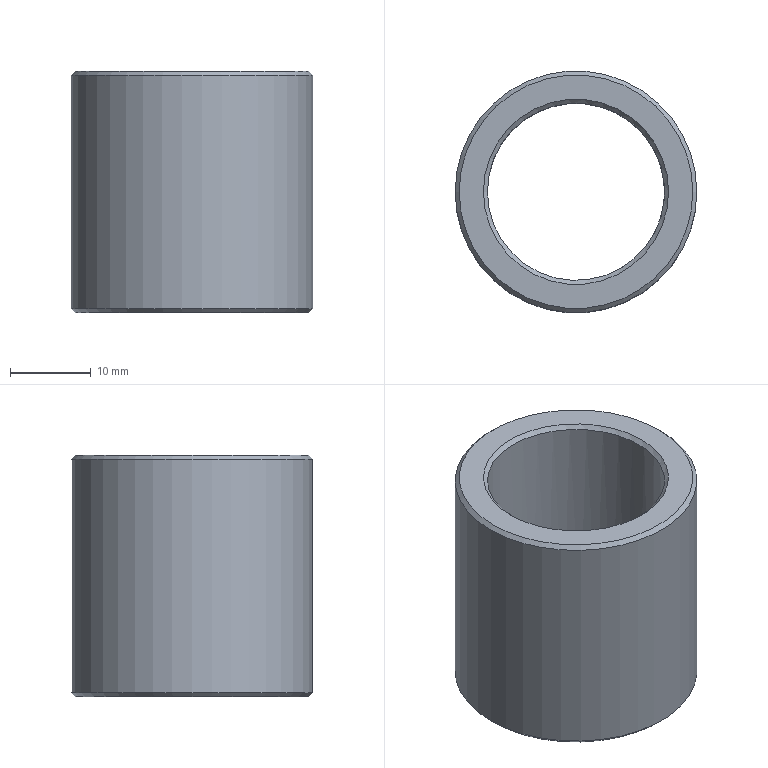Part | STEP file | solid 223 | 1 solid | 8 faces | box 30 x 30 x 30 mm | volume 9761 mm3 | cone 4 | plane 2 | cylinder 2 | commonest cylinder face diameters 22 x1 30 x1